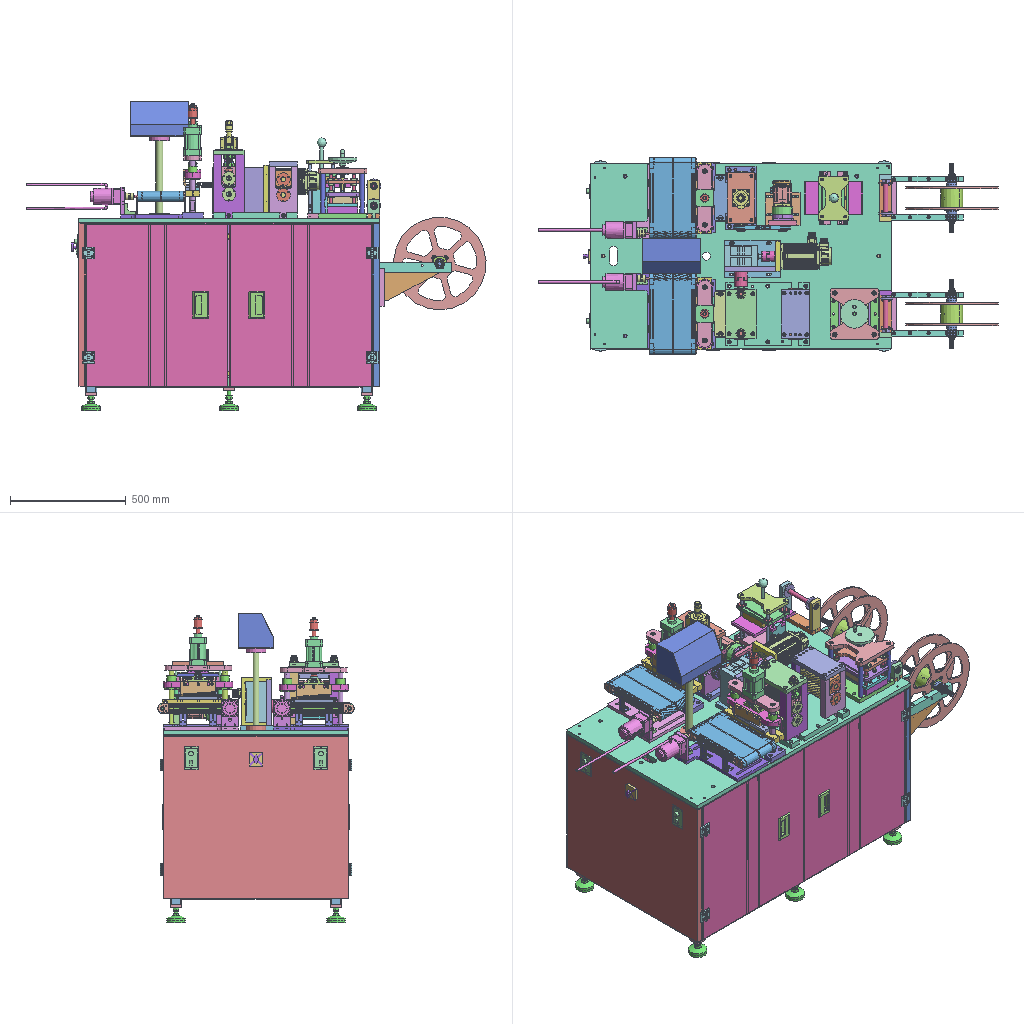Assembly | STEP file | 146 different items | 335 placed | box 1985 x 849 x 1335 mm
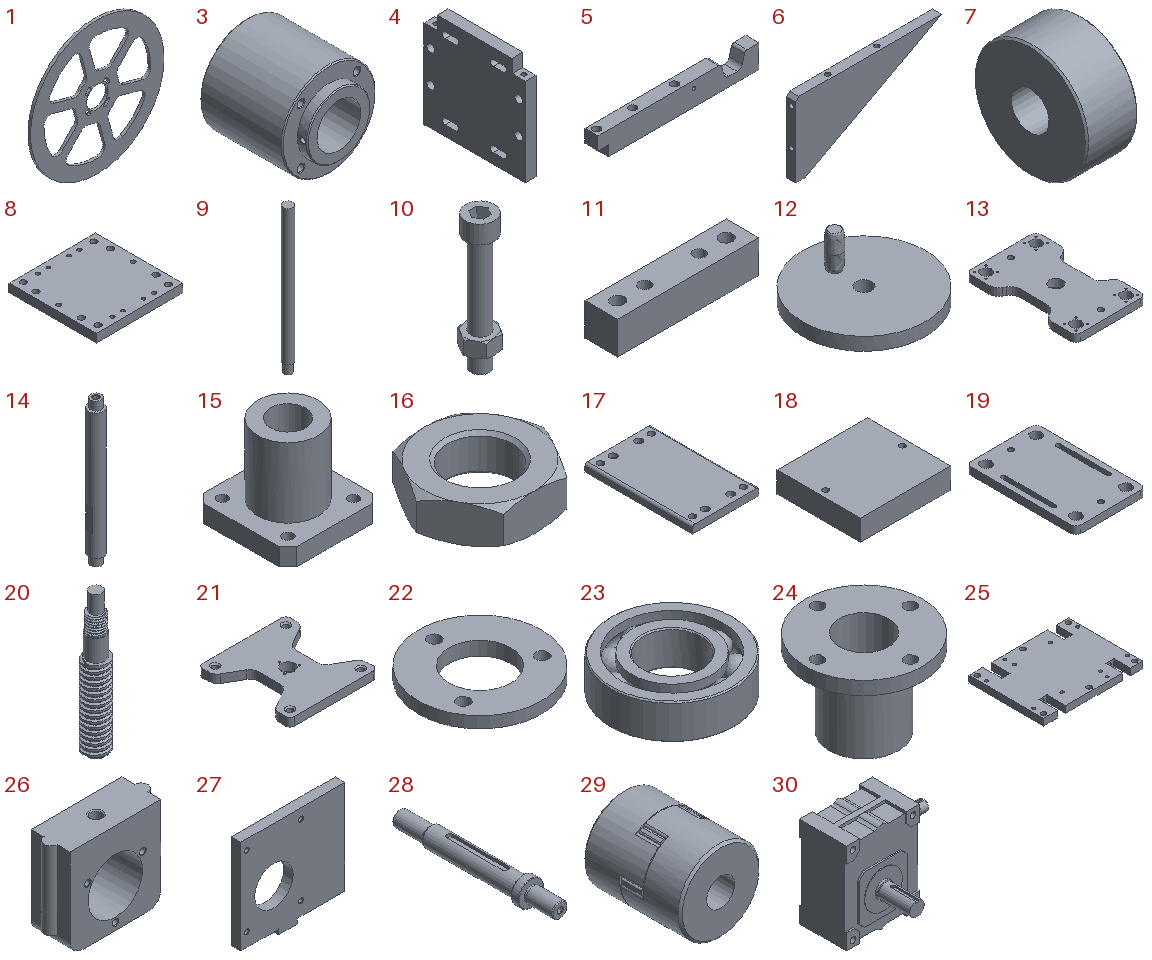Parts list (item | name | quantity | parent item | size | volume):
1 | YBQDJ-FLJ-1 | x4 | in YBQDJ-FLJ | 400 x 8 x 400 mm | 566908 mm3
2 | YBQDJ-FLJ-3 | x2 | in YBQDJ-FLJ | - | -
3 | YBQDJ-FLJ-2 | x2 | in YBQDJ-FLJ | 95 x 103 x 95 mm | 482469 mm3
4 | YBQDJ-FLJ-5 | x2 | in YBQDJ-FLJ | 20 x 190 x 190 mm | 661776 mm3
5 | YBQDJ-FLJ-4 | x4 | in YBQDJ-FLJ | 310 x 25 x 45 mm | 300462 mm3
6 | YBQDJ-FLJ-6 | x4 | in YBQDJ-FLJ | 237.857 x 15 x 120 mm | 224363 mm3
7 | YBQDJ-FLJ-7 | x8 | in YBQDJ-FLJ | 15 x 33 x 33 mm | 11378 mm3
8 | YBQDJ-YL-1 | x1 | in YBQDJ-YL | 210 x 210 x 20 mm | 848713 mm3
9 | YBQDJ-YL-8 | x4 | in YBQDJ-YL | 12 x 12 x 182 mm | 19664 mm3
10 | YBQDJ-YL-13 | x2 | in YBQDJ-YL | 18.475 x 16 x 75 mm | 8074 mm3
11 | YBQDJ-YL-2 | x2 | in YBQDJ-YL | 130 x 30 x 30 mm | 104775 mm3
12 | YBQDJ-YL-10 | x1 | in YBQDJ-YL | 125 x 125 x 70 mm | 226936 mm3
13 | YBQDJ-YL-5 | x1 | in YBQDJ-YL | 140 x 220 x 15 mm | 360572 mm3
14 | YBQDJ-YL-9 | x4 | in YBQDJ-YL | 20 x 20 x 198 mm | 57396 mm3
15 | YBQDJ-YL-14 | x8 | in YBQDJ-YL | 32 x 32 x 30 mm | 10494 mm3
16 | YBQDJ-YL-12 | x1 | in YBQDJ-YL | 24.249 x 21 x 7 mm | 1795 mm3
17 | YBQDJ-YL-3 | x1 | in YBQDJ-YL | 130 x 210 x 15 mm | 393827 mm3
18 | YBQDJ-YL-7 | x1 | in YBQDJ-YL | 130 x 120 x 30 mm | 464984 mm3
19 | YBQDJ-YL-4 | x1 | in YBQDJ-YL | 140 x 220 x 15 mm | 408740 mm3
20 | YBQDJ-YL-11 | x1 | in YBQDJ-YL | 20 x 20 x 118 mm | 24858 mm3
21 | YBQDJ-YL-6 | x1 | in YBQDJ-YL | 210 x 220 x 20 mm | 625567 mm3
22 | YBQDJ-YL-15 | x2 | in YBQDJ-YL | 54 x 54 x 6 mm | 8414 mm3
23 | YBQDJ-YL-16 | x2 | in YBQDJ-YL | 32 x 32 x 9 mm | 3911 mm3
24 | YBQDJ-YL-17 | x1 | in YBQDJ-YL | 44 x 44 x 32 mm | 13018 mm3
25 | YBQDJ-YB-1 | x1 | in YBQDJ-YB | 360 x 270 x 24 mm | 2084097 mm3
26 | YBQDJ-YB-3 | x2 | in YBQDJ-YB | 80 x 30 x 70 mm | 107518 mm3
27 | YBQDJ-YB-18 | x1 | in YBQDJ-YB | 220 x 20 x 210 mm | 773333 mm3
28 | YBQDJ-YB-16 | x1 | in YBQDJ-YB | 33 x 210 x 33 mm | 88192 mm3
29 | YBQDJ-YB-17 | x1 | in YBQDJ-YB | 55 x 66 x 55 mm | 122440 mm3
30 | YBQDJ-YB-20 | x1 | in YBQDJ-YB | 193 x 155 x 174 mm | 2083887 mm3
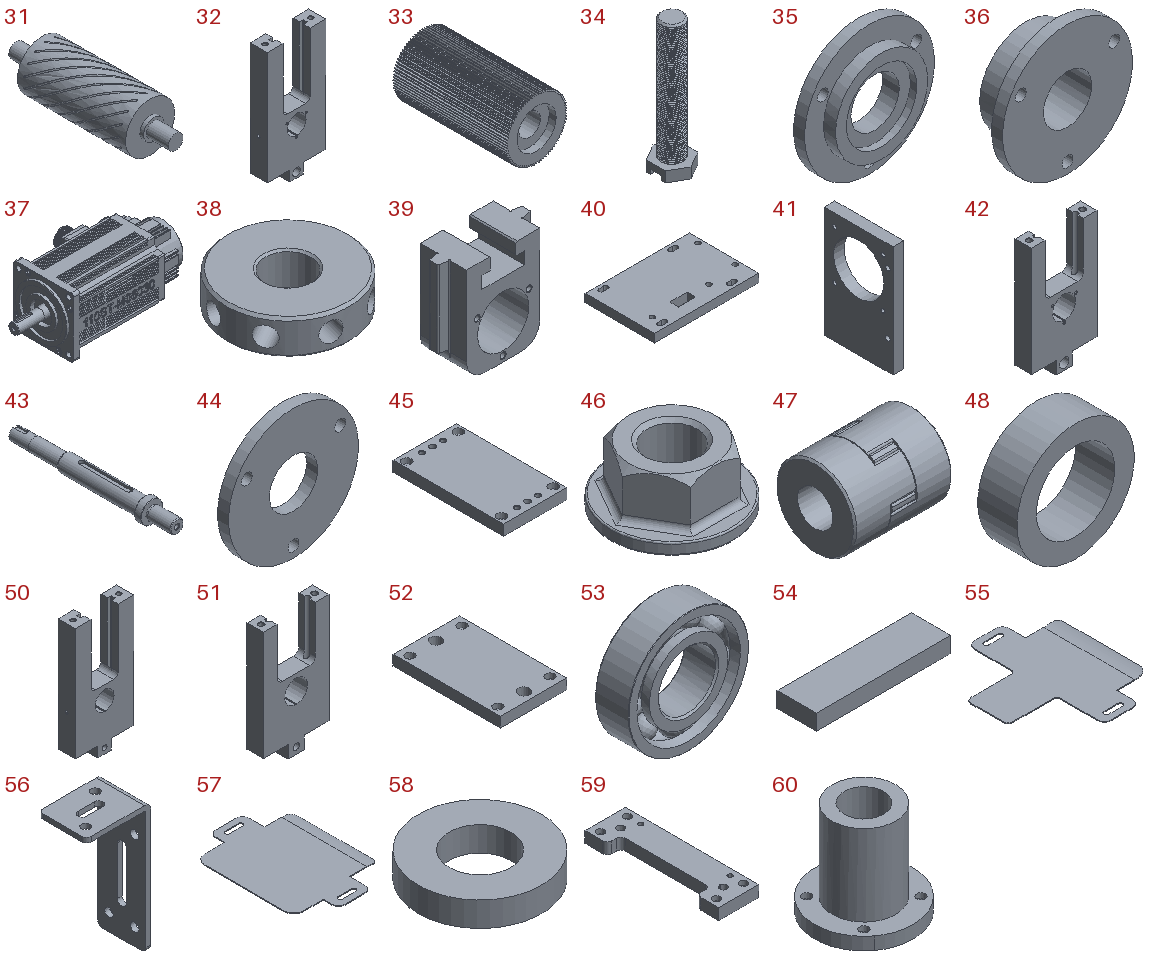31 | YBQDJ-YB-5 | x2 | in YBQDJ-YB | 68.992 x 218 x 68.953 mm | 543044 mm3
32 | YBQDJ-YB-6 | x1 | in YBQDJ-YB | 130 x 38 x 273 mm | 843391 mm3
33 | YBQDJ-YB-15 | x2 | in YBQDJ-YB | 69.832 x 130 x 69.818 mm | 396551 mm3
34 | YBQDJ-YB-8 | x2 | in YBQDJ-YB | 30 x 34.641 x 119.5 mm | 39653 mm3
35 | YBQDJ-YB-13 | x2 | in YBQDJ-YB | 59 x 10.5 x 59 mm | 15659 mm3
36 | YBQDJ-YB-12 | x2 | in YBQDJ-YB | 59 x 19 x 59 mm | 24092 mm3
37 | YBQDJ-YB-22 | x1 | in YBQDJ-YB | 275 x 158 x 110 mm | 3118501 mm3
38 | YBQDJ-YB-9 | x4 | in YBQDJ-YB | 50 x 50 x 14 mm | 18346 mm3
39 | YBQDJ-YB-7 | x2 | in YBQDJ-YB | 76 x 38 x 80 mm | 112101 mm3
40 | YBQDJ-YB-19 | x1 | in YBQDJ-YB | 240 x 160 x 19 mm | 686478 mm3
41 | YBQDJ-YB-21 | x1 | in YBQDJ-YB | 20 x 130 x 210 mm | 393461 mm3
42 | YBQDJ-YB-2 | x1 | in YBQDJ-YB | 120 x 30 x 223 mm | 466414 mm3
43 | YBQDJ-YB-11 | x1 | in YBQDJ-YB | 33 x 245 x 33 mm | 98573 mm3
44 | YBQDJ-YB-14 | x4 | in YBQDJ-YB | 59 x 5 x 59 mm | 11475 mm3
45 | YBQDJ-YB-4 | x1 | in YBQDJ-YB | 120 x 210 x 20 mm | 483124 mm3
46 | YBQDJ-YB-10 | x2 | in YBQDJ-YB | 42.8 x 42.8 x 20 mm | 13331 mm3
47 | YBQDJ-YB-23 | x1 | in YBQDJ-YB | 55 x 45 x 45 mm | 72571 mm3
48 | YBQDJ-YB-24 | x2 | in YBQDJ-YB | 30 x 10 x 30 mm | 3895 mm3
49 | YBQDJ-YB-25 | x1 | in YBQDJ-YB | - | -
50 | YBQDJ-YB-27 | x1 | in YBQDJ-YB | 130 x 38 x 273 mm | 843391 mm3
51 | YBQDJ-YB-26 | x1 | in YBQDJ-YB | 120 x 30 x 223 mm | 466414 mm3
52 | YBQDJ-YB-28 | x1 | in YBQDJ-YB | 130 x 210 x 20 mm | 518119 mm3
53 | YBQDJ-YB-29 | x16 | in YBQDJ-YB | 42 x 12 x 42 mm | 8686 mm3
54 | YBQDJ-YB-30 | x2 | in YBQDJ-YB | 34.5 x 10 x 4 mm | 1380 mm3
55 | YBQDJ-YB-34 | x1 | in YBQDJ-YB | 164.076 x 196 x 5.026 mm | 23129 mm3
56 | YBQDJ-YB-31 | x2 | in YBQDJ-YB | 40 x 30 x 80 mm | 9225 mm3
57 | YBQDJ-YB-32 | x1 | in YBQDJ-YB | 139.076 x 196 x 5.026 mm | 26086 mm3
58 | YBQDJ-YB-33 | x2 | in YBQDJ-YB | 20 x 20 x 4 mm | 942.478 mm3
59 | YBQDJ-QD-1 | x2 | in YBQDJ-QD-BD, YBQDJ-QD-PD | 90 x 300 x 25 mm | 495978 mm3
60 | YBQDJ-QD-7 | x4 | in YBQDJ-QD-BD, YBQDJ-QD-PD | 62 x 62 x 59 mm | 57722 mm3
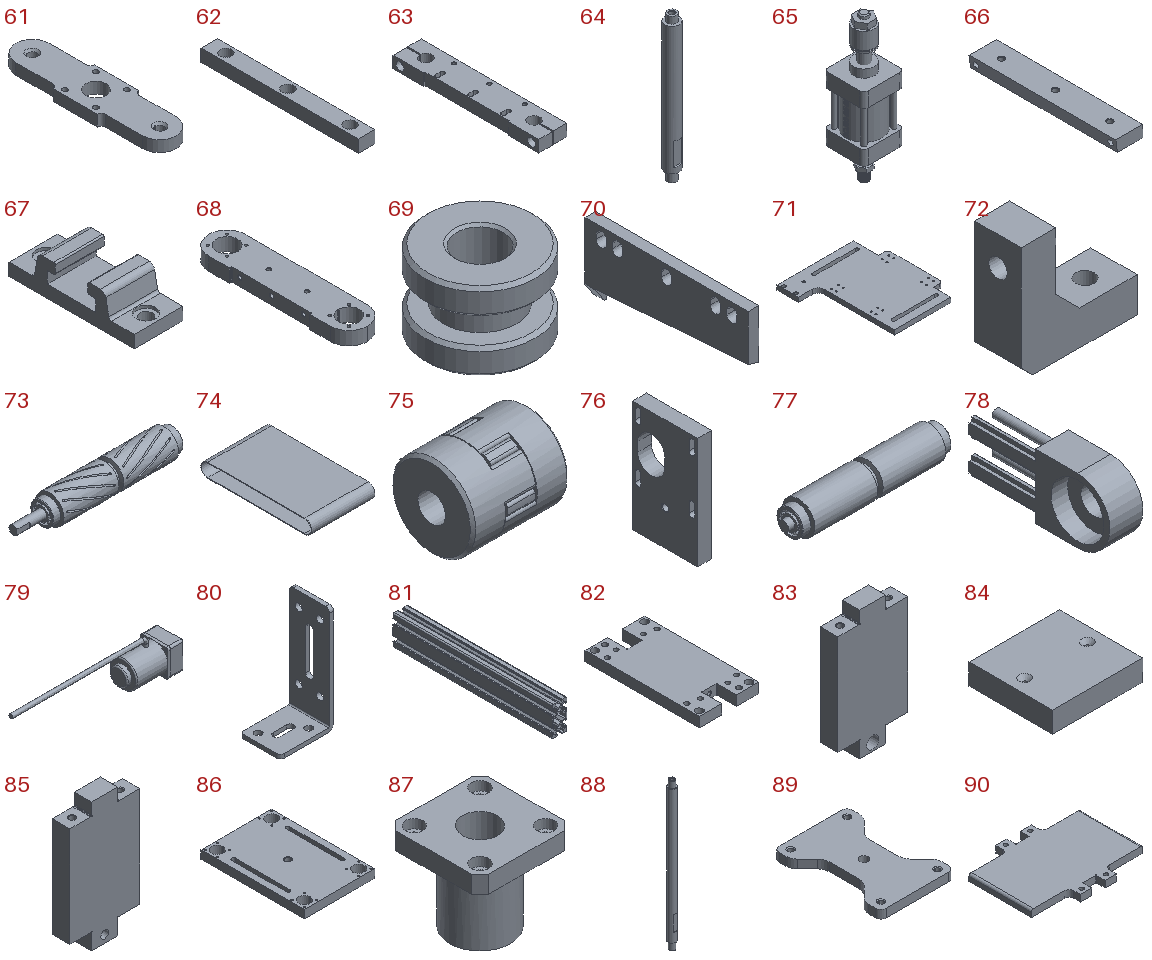61 | YBQDJ-QD-10 | x2 | in YBQDJ-QD-BD, YBQDJ-QD-PD | 75 x 290 x 20 mm | 318824 mm3
62 | YBQDJ-QD-4 | x2 | in YBQDJ-QD-BD, YBQDJ-QD-PD | 20 x 190 x 15 mm | 51822 mm3
63 | YBQDJ-QD-3 | x2 | in YBQDJ-QD-BD, YBQDJ-QD-PD | 60 x 310 x 25 mm | 397510 mm3
64 | YBQDJ-QD-2 | x2 | in YBQDJ-QD-BD | 25 x 25 x 254 mm | 111454 mm3
65 | YBQDJ-QD-11 | x2 | in YBQDJ-QD-BD, YBQDJ-QD-PD | 75 x 75 x 272 mm | 699847 mm3
66 | YBQDJ-QD-5 | x2 | in YBQDJ-QD-BD, YBQDJ-QD-PD | 35 x 190 x 15 mm | 92776 mm3
67 | YBQDJ-QD-8 | x2 | in YBQDJ-QD-BD, YBQDJ-QD-PD | 35 x 90 x 25 mm | 38677 mm3
68 | YBQDJ-QD-6 | x2 | in YBQDJ-QD-BD, YBQDJ-QD-PD | 70 x 300 x 25 mm | 414235 mm3
69 | YBQDJ-QD-9 | x2 | in YBQDJ-QD-BD, YBQDJ-QD-PD | 34 x 34 x 24 mm | 13509 mm3
70 | YBQDJ-QD-12 | x2 | in YBQDJ-QD-BD, YBQDJ-QD-PD | 10 x 150 x 65 mm | 69081 mm3
71 | YBQDJ-SSJ-1 | x1 | in YBQDJ-SSJ-BD | 280 x 320 x 15 mm | 982860 mm3
72 | YBQDJ-SSJ-8 | x2 | in YBQDJ-SSJ-BD, YBQD-SSJ-PD_MODEL | 50 x 20 x 50 mm | 24742 mm3
73 | YBQDJ-SSJ-7 | x2 | in YBQDJ-SSJ-BD, YBQD-SSJ-PD_MODEL | 227 x 40.957 x 41.285 mm | 212732 mm3
74 | YBQDJ-SSJ-3 | x2 | in YBQDJ-SSJ-BD, YBQD-SSJ-PD_MODEL | 200 x 350 x 44 mm | 311989 mm3
75 | YBQDJ-SSJ-11 | x2 | in YBQDJ-SSJ-BD, YBQD-SSJ-PD_MODEL | 35 x 30 x 30 mm | 20965 mm3
76 | YBQDJ-SSJ-9 | x2 | in YBQDJ-SSJ-BD, YBQD-SSJ-PD_MODEL | 15 x 70 x 120 mm | 105388 mm3
77 | YBQDJ-SSJ-6 | x2 | in YBQDJ-SSJ-BD, YBQD-SSJ-PD_MODEL | 196 x 40 x 40 mm | 211425 mm3
78 | YBQDJ-SSJ-4 | x8 | in YBQDJ-SSJ-BD, YBQD-SSJ-PD_MODEL | 20 x 85 x 39 mm | 27065 mm3
79 | YBQDJ-SSJ-10 | x2 | in YBQDJ-SSJ-BD, YBQD-SSJ-PD_MODEL | - | -
80 | YBQDJ-SSJ-2 | x8 | in YBQDJ-SSJ-BD, YBQD-SSJ-PD_MODEL | 40 x 30 x 80 mm | 9225 mm3
81 | YBQDJ-SSJ-5 | x4 | in YBQDJ-SSJ-BD, YBQD-SSJ-PD_MODEL | 20 x 215 x 40 mm | 63524 mm3
82 | YBQDJ-YY-1 | x1 | in YBQDJ-YY | 120 x 230 x 20 mm | 476492 mm3
83 | YBQDJ-YY-3 | x1 | in YBQDJ-YY | 80 x 20 x 148 mm | 197857 mm3
84 | YBQDJ-YY-5 | x1 | in YBQDJ-YY | 130 x 120 x 30 mm | 465920 mm3
85 | YBQDJ-YY-2 | x1 | in YBQDJ-YY | 80 x 20 x 148 mm | 197857 mm3
86 | YBQDJ-YY-7 | x1 | in YBQDJ-YY | 130 x 190 x 15 mm | 325427 mm3
87 | YBQDJ-YY-6 | x4 | in YBQDJ-YY | 32 x 32 x 30 mm | 10494 mm3
88 | YBQDJ-YY-10 | x4 | in YBQDJ-YY | 12 x 12 x 237 mm | 24995 mm3
89 | YBQDJ-YY-8 | x1 | in YBQDJ-YY | 130 x 190 x 15 mm | 272574 mm3
90 | YBQDJ-YY-4 | x1 | in YBQDJ-YY | 250 x 190 x 15 mm | 563148 mm3
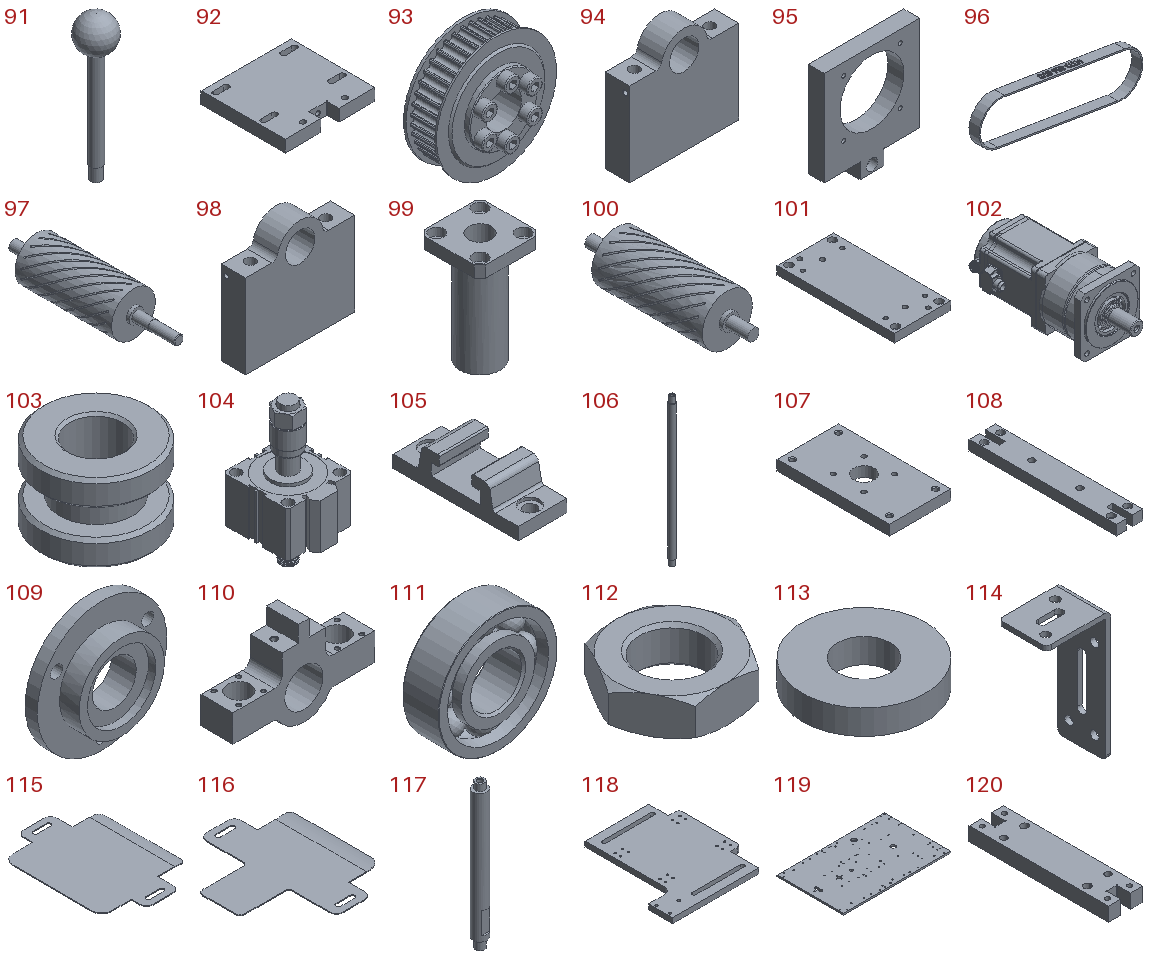91 | YBQDJ-YY-9 | x1 | in YBQDJ-YY | 40 x 40 x 166 mm | 52339 mm3
92 | YBQDJ-PD-1 | x1 | in YBQDJ-PD_MODEL | 150 x 140 x 20 mm | 385255 mm3
93 | YBQDJ-PD-4 | x2 | in YBQDJ-PD_MODEL | 67 x 28.5 x 67 mm | 55543 mm3
94 | YBQDJ-PD-7 | x1 | in YBQDJ-PD_MODEL | 130 x 29.2 x 127.5 mm | 362195 mm3
95 | YBQDJ-PD-3 | x1 | in YBQDJ-PD_MODEL | 120 x 20 x 138 mm | 191169 mm3
96 | YBQDJ-PD-5 | x1 | in YBQDJ-PD_MODEL | 245.482 x 15 x 95 mm | 17074 mm3
97 | YBQDJ-PD-9 | x1 | in YBQDJ-PD_MODEL | 68.992 x 253 x 68.953 mm | 537694 mm3
98 | YBQDJ-PD-8 | x1 | in YBQDJ-PD_MODEL | 130 x 29.2 x 127.5 mm | 362195 mm3
99 | YBQDJ-PD-11 | x4 | in YBQDJ-PD_MODEL | 32 x 32 x 57 mm | 16408 mm3
100 | YBQDJ-PD-10 | x1 | in YBQDJ-PD_MODEL | 68.992 x 218 x 68.953 mm | 532441 mm3
101 | YBQDJ-PD-6 | x1 | in YBQDJ-PD_MODEL | 130 x 270 x 19 mm | 640127 mm3
102 | YBQDJ-PD-2 | x1 | in YBQDJ-PD_MODEL | - | 675014 mm3
103 | YBQDJ-PD-16 | x1 | in YBQDJ-PD_MODEL | 34 x 34 x 24 mm | 12336 mm3
104 | YBQDJ-PD-15 | x1 | in YBQDJ-PD_MODEL | 76 x 84.5 x 162 mm | 333527 mm3
105 | YBQDJ-PD-17 | x1 | in YBQDJ-PD_MODEL | 35 x 90 x 25 mm | 38677 mm3
106 | YBQDJ-PD-13 | x4 | in YBQDJ-PD_MODEL | 12 x 12 x 284 mm | 30280 mm3
107 | YBQDJ-PD-14 | x1 | in YBQDJ-PD_MODEL | 120 x 220 x 20 mm | 489101 mm3
108 | YBQDJ-PD-18 | x1 | in YBQDJ-PD_MODEL | 40 x 220 x 15 mm | 117739 mm3
109 | YBQDJ-PD-19 | x4 | in YBQDJ-PD_MODEL | 53 x 13 x 53 mm | 13997 mm3
110 | YBQDJ-PD-12 | x2 | in YBQDJ-PD_MODEL | 130 x 29.2 x 80 mm | 97793 mm3
111 | YBQDJ-PD-20 | x8 | in YBQDJ-PD_MODEL | 35 x 11 x 35 mm | 5907 mm3
112 | YBQDJ-PD-21 | x1 | in YBQDJ-PD_MODEL | 31.177 x 27 x 9 mm | 3802 mm3
113 | YBQDJ-PD-24 | x2 | in YBQDJ-PD_MODEL | 20 x 20 x 4 mm | 1030 mm3
114 | YBQDJ-PD-25 | x2 | in YBQDJ-PD_MODEL | 40 x 30 x 80 mm | 9225 mm3
115 | YBQDJ-PD-22 | x1 | in YBQDJ-PD_MODEL | 139.076 x 196 x 5.026 mm | 26086 mm3
116 | YBQDJ-PD-23 | x1 | in YBQDJ-PD_MODEL | 164.076 x 196 x 5.026 mm | 23129 mm3
117 | YBQDJ-QD-PD-2 | x2 | in YBQDJ-QD-PD | 25 x 25 x 264 mm | 116363 mm3
118 | YBQDJ-SSJ-PD-1 | x1 | in YBQD-SSJ-PD_MODEL | 280 x 320 x 15 mm | 982860 mm3
119 | YBQDJ-Large plate | x1 | in Pressure-wave cutting all-in-one machine general unit | 1300 x 800 x 20 mm | 20508106 mm3
120 | YBQDJ-DX-1 | x2 | in YBQDJ-DX-PD_MODEL, YBQDJ-DX-BD_MODEL | 50 x 200 x 20 mm | 177964 mm3
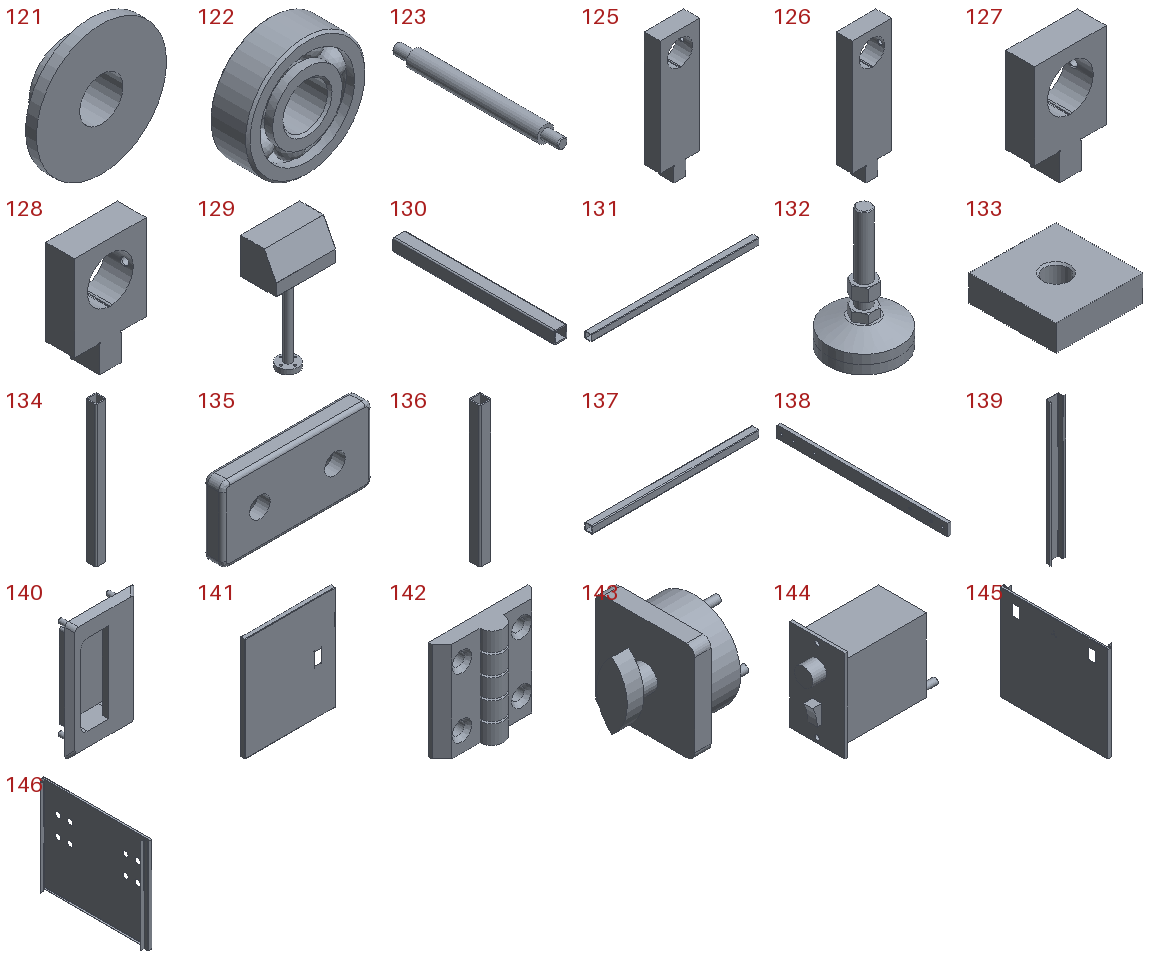121 | YBQDJ-DX-3 | x4 | in YBQDJ-DX-PD_MODEL, YBQDJ-DX-BD_MODEL | 60 x 16 x 60 mm | 19587 mm3
122 | YBQDJ-DX-6 | x8 | in YBQDJ-DX-PD_MODEL, YBQDJ-DX-BD_MODEL | 32 x 10 x 32 mm | 4745 mm3
123 | YBQDJ-DX-4 | x2 | in YBQDJ-DX-PD_MODEL, YBQDJ-DX-BD_MODEL | 20 x 200 x 20 mm | 54352 mm3
124 | YBQDJ-DX-5 | x2 | in YBQDJ-DX-PD_MODEL, YBQDJ-DX-BD_MODEL | - | -
125 | YBQDJ-DX-2 | x1 | in YBQDJ-DX-PD_MODEL | 50 x 20 x 164 mm | 134384 mm3
126 | YBQDJ-DX-7 | x1 | in YBQDJ-DX-PD_MODEL | 50 x 20 x 164 mm | 134384 mm3
127 | YBQDJ-DX-BD-2 | x1 | in YBQDJ-DX-BD_MODEL | 50 x 20 x 79 mm | 49384 mm3
128 | YBQDJ-DX-BD-7 | x1 | in YBQDJ-DX-BD_MODEL | 50 x 20 x 79 mm | 49384 mm3
129 | Touch screen assembly | x1 | in Pressure-wave cutting all-in-one machine general unit | 250 x 150 x 505 mm | 675168 mm3
130 | 50x50x640 | x6 | in YBQDJ-JJ_MODEL | 50 x 640 x 50 mm | 562265 mm3
131 | 50x50x1240 | x2 | in YBQDJ-JJ_MODEL | 1240 x 50 x 50 mm | 1089389 mm3
132 | Foot cup | x6 | in 50x50x680_MODEL, 50x50x1140_MODEL | 80 x 80 x 135 mm | 154518 mm3
133 | Pad block | x6 | in 50x50x680_MODEL, 50x50x1140_MODEL | 50 x 50 x 15 mm | 35145 mm3
134 | SOLID | x4 | in 50x50x680_MODEL | 50 x 50 x 680 mm | 597407 mm3
135 | Door magnet | x4 | in 50x50x610_MODEL | 40 x 5 x 20 mm | 3632 mm3
136 | SOLID | x2 | in 50x50x610_MODEL | 50 x 50 x 610 mm | 535909 mm3
137 | SOLID | x2 | in 50x50x1140_MODEL | 1140 x 50 x 50 mm | 1000530 mm3
138 | Crossbeam | x2 | in YBQDJ-JJ_MODEL | 15 x 730 x 50 mm | 541334 mm3
139 | Reinforcing rib | x4 | in YBQDJ-BJ-1_MODEL | 80 x 26.7 x 696 mm | 106400 mm3
140 | Handle | x4 | in YBQDJ-BJ-1_MODEL | 69 x 21 x 119 mm | 44051 mm3
141 | SOLID | x4 | in YBQDJ-BJ-1_MODEL | 615 x 30 x 705 mm | 627775 mm3
142 | Hinge | x8 | in YBQDJ-BJ_MODEL | 50 x 12.7 x 49.8 mm | 17221 mm3
143 | Power switch | x1 | in YBQDJ-BJ-2_MODEL | 64 x 60 x 60 mm | 180692 mm3
144 | Speed control panel | x2 | in YBQDJ-BJ-2_MODEL | 122.5 x 60 x 100 mm | 404808 mm3
145 | SOLID | x1 | in YBQDJ-BJ-2_MODEL | 55 x 800 x 705 mm | 825706 mm3
146 | YBQDJ-BJ-3 | x1 | in YBQDJ-BJ_MODEL | 55 x 800 x 705 mm | 823970 mm3
Placements (level | parent | child | x y z in mm | rotation matrix by rows), first 235 of 362 lines:
1 | Pressure-wave cutting all-in-one machine general unit | YBQDJ-FLJ | 0.0 0.0 0.0 | 1 0 0 0 1 0 0 0 1
2 | YBQDJ-FLJ | YBQDJ-FLJ-1 | 0.0 0.0 0.0 | 1 0 0 0 1 0 0 0 1
2 | YBQDJ-FLJ | YBQDJ-FLJ-3 | 0.0 0.0 0.0 | 1 0 0 0 1 0 0 0 1
2 | YBQDJ-FLJ | YBQDJ-FLJ-2 | 0.0 0.0 0.0 | 1 0 0 0 1 0 0 0 1
2 | YBQDJ-FLJ | YBQDJ-FLJ-1 | 0.0 91.0 0.0 | 1 0 0 0 1 0 0 0 1
2 | YBQDJ-FLJ | YBQDJ-FLJ-5 | 0.0 0.0 0.0 | 1 0 0 0 1 0 0 0 1
2 | YBQDJ-FLJ | YBQDJ-FLJ-4 | 0.0 0.0 0.0 | 1 0 0 0 1 0 0 0 1
2 | YBQDJ-FLJ | YBQDJ-FLJ-6 | 0.0 0.0 0.0 | 1 0 0 0 1 0 0 0 1
2 | YBQDJ-FLJ | YBQDJ-FLJ-6 | 0.0 165.0 0.0 | 1 0 0 0 1 0 0 0 1
2 | YBQDJ-FLJ | YBQDJ-FLJ-4 | 0.0 165.0 0.0 | 1 0 0 0 1 0 0 0 1
2 | YBQDJ-FLJ | YBQDJ-FLJ-7 | -0.0 90.0 -140.0 | 1 0 0 0 1 0 0 0 1
2 | YBQDJ-FLJ | YBQDJ-FLJ-7 | -0.0 90.0 -0.0 | 1 0 0 0 1 0 0 0 1
2 | YBQDJ-FLJ | YBQDJ-FLJ-7 | 0.0 0.0 0.0 | 1 0 0 0 1 0 0 0 1
2 | YBQDJ-FLJ | YBQDJ-FLJ-7 | 0.0 0.0 -140.0 | 1 0 0 0 1 0 0 0 1
1 | Pressure-wave cutting all-in-one machine general unit | YBQDJ-FLJ | 0.0 500.0 0.0 | 1 0 0 0 1 0 0 0 1
2 | YBQDJ-FLJ | YBQDJ-FLJ-1 | 0.0 0.0 0.0 | 1 0 0 0 1 0 0 0 1
2 | YBQDJ-FLJ | YBQDJ-FLJ-3 | 0.0 0.0 0.0 | 1 0 0 0 1 0 0 0 1
2 | YBQDJ-FLJ | YBQDJ-FLJ-2 | 0.0 0.0 0.0 | 1 0 0 0 1 0 0 0 1
2 | YBQDJ-FLJ | YBQDJ-FLJ-1 | 0.0 91.0 0.0 | 1 0 0 0 1 0 0 0 1
2 | YBQDJ-FLJ | YBQDJ-FLJ-5 | 0.0 0.0 0.0 | 1 0 0 0 1 0 0 0 1
2 | YBQDJ-FLJ | YBQDJ-FLJ-4 | 0.0 0.0 0.0 | 1 0 0 0 1 0 0 0 1
2 | YBQDJ-FLJ | YBQDJ-FLJ-6 | 0.0 0.0 0.0 | 1 0 0 0 1 0 0 0 1
2 | YBQDJ-FLJ | YBQDJ-FLJ-6 | 0.0 165.0 0.0 | 1 0 0 0 1 0 0 0 1
2 | YBQDJ-FLJ | YBQDJ-FLJ-4 | 0.0 165.0 0.0 | 1 0 0 0 1 0 0 0 1
2 | YBQDJ-FLJ | YBQDJ-FLJ-7 | -0.0 90.0 -140.0 | 1 0 0 0 1 0 0 0 1
2 | YBQDJ-FLJ | YBQDJ-FLJ-7 | -0.0 90.0 -0.0 | 1 0 0 0 1 0 0 0 1
2 | YBQDJ-FLJ | YBQDJ-FLJ-7 | 0.0 0.0 0.0 | 1 0 0 0 1 0 0 0 1
2 | YBQDJ-FLJ | YBQDJ-FLJ-7 | 0.0 0.0 -140.0 | 1 0 0 0 1 0 0 0 1
1 | Pressure-wave cutting all-in-one machine general unit | YBQDJ-YL | 0.0 0.0 0.0 | 1 0 0 0 1 0 0 0 1
2 | YBQDJ-YL | YBQDJ-YL-1 | 0.0 0.0 0.0 | 1 0 0 0 1 0 0 0 1
2 | YBQDJ-YL | YBQDJ-YL-8 | 0.0 0.0 0.0 | 1 0 0 0 1 0 0 0 1
2 | YBQDJ-YL | YBQDJ-YL-13 | 0.0 0.0 0.0 | 1 0 0 0 1 0 0 0 1
2 | YBQDJ-YL | YBQDJ-YL-2 | 0.0 0.0 0.0 | 1 0 0 0 1 0 0 0 1
2 | YBQDJ-YL | YBQDJ-YL-10 | 0.0 0.0 0.0 | 1 0 0 0 1 0 0 0 1
2 | YBQDJ-YL | YBQDJ-YL-5 | 0.0 0.0 0.0 | 1 0 0 0 1 0 0 0 1
2 | YBQDJ-YL | YBQDJ-YL-9 | 0.0 0.0 0.0 | 1 0 0 0 1 0 0 0 1
2 | YBQDJ-YL | YBQDJ-YL-14 | 0.0 0.0 0.0 | 1 0 0 0 1 0 0 0 1
2 | YBQDJ-YL | YBQDJ-YL-12 | 0.0 0.0 0.5 | 1 0 0 0 1 0 0 0 1
2 | YBQDJ-YL | YBQDJ-YL-3 | 0.0 0.0 0.0 | 1 0 0 0 1 0 0 0 1
2 | YBQDJ-YL | YBQDJ-YL-7 | 0.0 0.0 0.0 | 1 0 0 0 1 0 0 0 1
2 | YBQDJ-YL | YBQDJ-YL-4 | 0.0 0.0 0.0 | 1 0 0 0 1 0 0 0 1
2 | YBQDJ-YL | YBQDJ-YL-11 | 0.0 0.0 0.0 | 1 0 0 0 1 0 0 0 1
2 | YBQDJ-YL | YBQDJ-YL-6 | 0.0 0.0 0.0 | 1 0 0 0 1 0 0 0 1
2 | YBQDJ-YL | YBQDJ-YL-2 | 0.0 180.0 0.0 | 1 0 0 0 1 0 0 0 1
2 | YBQDJ-YL | YBQDJ-YL-14 | 100.0 0.0 0.0 | 1 0 0 0 1 0 0 0 1
2 | YBQDJ-YL | YBQDJ-YL-14 | 100.0 180.0 0.0 | 1 0 0 0 1 0 0 0 1
2 | YBQDJ-YL | YBQDJ-YL-14 | 0.0 180.0 0.0 | 1 0 0 0 1 0 0 0 1
2 | YBQDJ-YL | YBQDJ-YL-14 | 613.0 0.0 260.0 | -1 0 0 0 1 0 0 0 -1
2 | YBQDJ-YL | YBQDJ-YL-14 | 513.0 0.0 260.0 | -1 0 0 0 1 0 0 0 -1
2 | YBQDJ-YL | YBQDJ-YL-14 | 613.0 180.0 260.0 | -1 0 0 0 1 0 0 0 -1
2 | YBQDJ-YL | YBQDJ-YL-14 | 513.0 180.0 260.0 | -1 0 0 0 1 0 0 0 -1
2 | YBQDJ-YL | YBQDJ-YL-13 | 0.0 180.0 0.0 | 1 0 0 0 1 0 0 0 1
2 | YBQDJ-YL | YBQDJ-YL-8 | 100.0 0.0 0.0 | 1 0 0 0 1 0 0 0 1
2 | YBQDJ-YL | YBQDJ-YL-8 | 0.0 180.0 0.0 | 1 0 0 0 1 0 0 0 1
2 | YBQDJ-YL | YBQDJ-YL-8 | 100.0 180.0 0.0 | 1 0 0 0 1 0 0 0 1
2 | YBQDJ-YL | YBQDJ-YL-9 | 170.0 0.0 0.0 | 1 0 0 0 1 0 0 0 1
2 | YBQDJ-YL | YBQDJ-YL-9 | 170.0 180.0 0.0 | 1 0 0 0 1 0 0 0 1
2 | YBQDJ-YL | YBQDJ-YL-9 | 0.0 180.0 0.0 | 1 0 0 0 1 0 0 0 1
2 | YBQDJ-YL | YBQDJ-YL-15 | 0.0 0.0 0.0 | 1 0 0 0 1 0 0 0 1
2 | YBQDJ-YL | YBQDJ-YL-16 | 0.0 0.0 0.0 | 1 0 0 0 1 0 0 0 1
2 | YBQDJ-YL | YBQDJ-YL-17 | 0.0 0.0 0.0 | 1 0 0 0 1 0 0 0 1
2 | YBQDJ-YL | YBQDJ-YL-16 | 0.0 0.0 9.0 | 1 0 0 0 1 0 0 0 1
2 | YBQDJ-YL | YBQDJ-YL-15 | 613.0 0.0 408.0 | -1 0 0 0 1 0 0 0 -1
1 | Pressure-wave cutting all-in-one machine general unit | YBQDJ-YB | 0.0 0.0 0.0 | 1 0 0 0 1 0 0 0 1
2 | YBQDJ-YB | YBQDJ-YB-1 | 0.0 0.0 0.0 | 1 0 0 0 1 0 0 0 1
2 | YBQDJ-YB | YBQDJ-YB-3 | 0.0 0.0 0.0 | 1 0 0 0 1 0 0 0 1
2 | YBQDJ-YB | YBQDJ-YB-18 | 0.0 0.0 0.0 | 1 0 0 0 1 0 0 0 1
2 | YBQDJ-YB | YBQDJ-YB-16 | 0.0 0.0 0.0 | 1 0 0 0 1 0 0 0 1
2 | YBQDJ-YB | YBQDJ-YB-17 | 0.0 0.0 0.0 | 1 0 0 0 1 0 0 0 1
2 | YBQDJ-YB | YBQDJ-YB-20 | 0.0 0.0 0.0 | 1 0 0 0 1 0 0 0 1
2 | YBQDJ-YB | YBQDJ-YB-5 | 0.0 0.0 0.0 | 1 0 0 0 1 0 0 0 1
2 | YBQDJ-YB | YBQDJ-YB-6 | 0.0 0.0 0.0 | 1 0 0 0 1 0 0 0 1
2 | YBQDJ-YB | YBQDJ-YB-15 | 0.0 0.0 0.0 | 1 0 0 0 1 0 0 0 1
2 | YBQDJ-YB | YBQDJ-YB-8 | 0.0 0.0 0.0 | 1 0 0 0 1 0 0 0 1
2 | YBQDJ-YB | YBQDJ-YB-13 | 0.0 0.0 0.0 | 1 0 0 0 1 0 0 0 1
2 | YBQDJ-YB | YBQDJ-YB-12 | 0.0 0.0 0.0 | 1 0 0 0 1 0 0 0 1
2 | YBQDJ-YB | YBQDJ-YB-22 | 0.0 0.0 0.0 | 1 0 0 0 1 0 0 0 1
2 | YBQDJ-YB | YBQDJ-YB-9 | 0.0 0.0 0.0 | 1 0 0 0 1 0 0 0 1
2 | YBQDJ-YB | YBQDJ-YB-7 | 0.0 0.0 0.0 | 1 0 0 0 1 0 0 0 1
2 | YBQDJ-YB | YBQDJ-YB-19 | 0.0 0.0 0.0 | 1 0 0 0 1 0 0 0 1
2 | YBQDJ-YB | YBQDJ-YB-21 | 0.0 0.0 0.0 | 1 0 0 0 1 0 0 0 1
2 | YBQDJ-YB | YBQDJ-YB-2 | 0.0 0.0 0.0 | 1 0 0 0 1 0 0 0 1
2 | YBQDJ-YB | YBQDJ-YB-11 | 0.0 0.0 0.0 | 1 0 0 0 1 0 0 0 1
2 | YBQDJ-YB | YBQDJ-YB-14 | 0.0 0.0 0.0 | 1 0 0 0 1 0 0 0 1
2 | YBQDJ-YB | YBQDJ-YB-4 | 0.0 0.0 0.0 | 1 0 0 0 1 0 0 0 1
2 | YBQDJ-YB | YBQDJ-YB-10 | 0.0 0.0 0.0 | 1 0 0 0 1 0 0 0 1
2 | YBQDJ-YB | YBQDJ-YB-23 | 0.0 0.0 0.0 | 1 0 0 0 1 0 0 0 1
2 | YBQDJ-YB | YBQDJ-YB-24 | 0.0 0.0 0.0 | 1 0 0 0 1 0 0 0 1
2 | YBQDJ-YB | YBQDJ-YB-25 | 0.0 0.0 0.0 | 1 0 0 0 1 0 0 0 1
2 | YBQDJ-YB | YBQDJ-YB-27 | 0.0 0.0 0.0 | 1 0 0 0 1 0 0 0 1
2 | YBQDJ-YB | YBQDJ-YB-26 | 0.0 0.0 0.0 | 1 0 0 0 1 0 0 0 1
2 | YBQDJ-YB | YBQDJ-YB-28 | 0.0 0.0 0.0 | 1 0 0 0 1 0 0 0 1
2 | YBQDJ-YB | YBQDJ-YB-29 | 0.0 0.0 0.0 | 1 0 0 0 1 0 0 0 1
2 | YBQDJ-YB | YBQDJ-YB-29 | 0.0 -12.0 0.0 | 1 0 0 0 1 0 0 0 1
2 | YBQDJ-YB | YBQDJ-YB-29 | 0.0 182.0 0.0 | 1 0 0 0 1 0 0 0 1
2 | YBQDJ-YB | YBQDJ-YB-29 | 0.0 170.0 0.0 | 1 0 0 0 1 0 0 0 1
2 | YBQDJ-YB | YBQDJ-YB-29 | 0.0 0.0 67.0 | 1 0 0 0 1 0 0 0 1
2 | YBQDJ-YB | YBQDJ-YB-29 | 0.0 170.0 67.0 | 1 0 0 0 1 0 0 0 1
2 | YBQDJ-YB | YBQDJ-YB-29 | 0.0 182.0 67.0 | 1 0 0 0 1 0 0 0 1
2 | YBQDJ-YB | YBQDJ-YB-5 | 0.0 0.0 67.0 | 1 0 0 0 1 0 0 0 1
2 | YBQDJ-YB | YBQDJ-YB-29 | 0.0 -12.0 67.0 | 1 0 0 0 1 0 0 0 1
2 | YBQDJ-YB | YBQDJ-YB-14 | -0.0 0.0 67.0 | 1 0 0 0 1 0 0 0 1
2 | YBQDJ-YB | YBQDJ-YB-3 | 103.0 -390.0 0.0 | -1 0 0 0 -1 0 0 0 1
2 | YBQDJ-YB | YBQDJ-YB-14 | 103.0 -390.0 0.0 | -1 0 0 0 -1 0 0 0 1
2 | YBQDJ-YB | YBQDJ-YB-14 | 103.0 -390.0 67.0 | -1 0 0 0 -1 0 0 0 1
2 | YBQDJ-YB | YBQDJ-YB-15 | 0.0 0.0 68.3 | 1 0 0 0 1 0 0 0 1
2 | YBQDJ-YB | YBQDJ-YB-29 | -235.0 12.0 3.0 | 1 0 0 0 1 0 0 0 1
2 | YBQDJ-YB | YBQDJ-YB-29 | -235.0 0.0 3.0 | 1 0 0 0 1 0 0 0 1
2 | YBQDJ-YB | YBQDJ-YB-29 | -235.0 0.0 71.3 | 1 0 0 0 1 0 0 0 1
2 | YBQDJ-YB | YBQDJ-YB-29 | -235.0 12.0 71.3 | 1 0 0 0 1 0 0 0 1
2 | YBQDJ-YB | YBQDJ-YB-12 | -0.0 0.0 68.3 | 1 0 0 0 1 0 0 0 1
2 | YBQDJ-YB | YBQDJ-YB-9 | 0.0 0.0 36.7 | 1 0 0 0 1 0 0 0 1
2 | YBQDJ-YB | YBQDJ-YB-7 | -367 -390 -0.0 | -1 1e-06 0 -1e-06 -1 0 0 0 1
2 | YBQDJ-YB | YBQDJ-YB-9 | 0.0 172.0 36.7 | 1 0 0 0 1 0 0 0 1
2 | YBQDJ-YB | YBQDJ-YB-8 | 0.0 172.0 0.0 | 1 0 0 0 1 0 0 0 1
2 | YBQDJ-YB | YBQDJ-YB-9 | 0.0 172.0 0.0 | 1 0 0 0 1 0 0 0 1
2 | YBQDJ-YB | YBQDJ-YB-10 | 0.0 172.0 0.0 | 1 0 0 0 1 0 0 0 1
2 | YBQDJ-YB | YBQDJ-YB-24 | 0.0 0.0 68.3 | 1 0 0 0 1 0 0 0 1
2 | YBQDJ-YB | YBQDJ-YB-29 | -235.0 166.5 3.0 | 1 0 0 0 1 0 0 0 1
2 | YBQDJ-YB | YBQDJ-YB-29 | -235.0 178.5 3.0 | 1 0 0 0 1 0 0 0 1
2 | YBQDJ-YB | YBQDJ-YB-13 | 0.0 0.0 68.3 | 1 0 0 0 1 0 0 0 1
2 | YBQDJ-YB | YBQDJ-YB-29 | -235.0 178.5 71.3 | 1 0 0 0 1 0 0 0 1
2 | YBQDJ-YB | YBQDJ-YB-29 | -235.0 166.5 71.3 | 1 0 0 0 1 0 0 0 1
2 | YBQDJ-YB | YBQDJ-YB-30 | 0.0 172.0 0.0 | 1 0 0 0 1 0 0 0 1
2 | YBQDJ-YB | YBQDJ-YB-30 | 0.0 0.0 0.0 | 1 0 0 0 1 0 0 0 1
2 | YBQDJ-YB | YBQDJ-YB-34 | 0.0 0.0 0.0 | 1 0 0 0 1 0 0 0 1
2 | YBQDJ-YB | YBQDJ-YB-31 | 0.0 0.0 0.0 | 1 0 0 0 1 0 0 0 1
2 | YBQDJ-YB | YBQDJ-YB-32 | -0.5 0.0 0.0 | 1 0 0 0 1 0 0 0 1
2 | YBQDJ-YB | YBQDJ-YB-33 | 0.0 0.0 0.0 | 1 0 0 0 1 0 0 0 1
2 | YBQDJ-YB | YBQDJ-YB-31 | 0.0 172.0 0.0 | 1 0 0 0 1 0 0 0 1
2 | YBQDJ-YB | YBQDJ-YB-33 | 0.0 172.0 0.0 | 1 0 0 0 1 0 0 0 1
1 | Pressure-wave cutting all-in-one machine general unit | YBQDJ-QD-BD | 0.0 0.0 0.0 | 1 0 0 0 1 0 0 0 1
2 | YBQDJ-QD-BD | YBQDJ-QD-1 | 0.0 0.0 0.0 | 1 0 0 0 1 0 0 0 1
2 | YBQDJ-QD-BD | YBQDJ-QD-7 | 0.0 0.0 0.0 | 1 0 0 0 1 0 0 0 1
2 | YBQDJ-QD-BD | YBQDJ-QD-10 | 0.0 0.0 0.0 | 1 0 0 0 1 0 0 0 1
2 | YBQDJ-QD-BD | YBQDJ-QD-4 | 0.0 0.0 0.0 | 1 0 0 0 1 0 0 0 1
2 | YBQDJ-QD-BD | YBQDJ-QD-3 | 0.0 0.0 0.0 | 1 0 0 0 1 0 0 0 1
2 | YBQDJ-QD-BD | YBQDJ-QD-2 | 0.0 0.0 0.0 | 1 0 0 0 1 0 0 0 1
2 | YBQDJ-QD-BD | YBQDJ-QD-11 | 0.0 0.0 0.0 | 1 0 0 0 1 0 0 0 1
2 | YBQDJ-QD-BD | YBQDJ-QD-5 | 0.0 0.0 0.0 | 1 0 0 0 1 0 0 0 1
2 | YBQDJ-QD-BD | YBQDJ-QD-8 | 0.0 0.0 0.0 | 1 0 0 0 1 0 0 0 1
2 | YBQDJ-QD-BD | YBQDJ-QD-6 | 0.0 0.0 0.0 | 1 0 0 0 1 0 0 0 1
2 | YBQDJ-QD-BD | YBQDJ-QD-9 | 0.0 0.0 0.0 | 1 0 0 0 1 0 0 0 1
2 | YBQDJ-QD-BD | YBQDJ-QD-12 | 0.0 0.0 0.0 | 1 0 0 0 1 0 0 0 1
2 | YBQDJ-QD-BD | YBQDJ-QD-2 | 0.0 230.0 0.0 | 1 0 0 0 1 0 0 0 1
2 | YBQDJ-QD-BD | YBQDJ-QD-7 | 0.0 230.0 0.0 | 1 0 0 0 1 0 0 0 1
1 | Pressure-wave cutting all-in-one machine general unit | YBQDJ-SSJ-BD | 0.0 0.0 0.0 | 1 0 0 0 1 0 0 0 1
2 | YBQDJ-SSJ-BD | YBQDJ-SSJ-1 | 0.0 0.0 0.0 | 1 0 0 0 1 0 0 0 1
2 | YBQDJ-SSJ-BD | YBQDJ-SSJ-8 | 0.0 0.0 0.0 | 1 0 0 0 1 0 0 0 1
2 | YBQDJ-SSJ-BD | YBQDJ-SSJ-7 | 0.0 0.0 0.0 | 1 0 0 0 1 0 0 0 1
2 | YBQDJ-SSJ-BD | YBQDJ-SSJ-3 | 0.0 0.0 0.0 | 1 0 0 0 1 0 0 0 1
2 | YBQDJ-SSJ-BD | YBQDJ-SSJ-11 | 0.0 0.0 0.0 | 1 0 0 0 1 0 0 0 1
2 | YBQDJ-SSJ-BD | YBQDJ-SSJ-9 | 0.0 0.0 0.0 | 1 0 0 0 1 0 0 0 1
2 | YBQDJ-SSJ-BD | YBQDJ-SSJ-6 | 0.0 0.0 0.0 | 1 0 0 0 1 0 0 0 1
2 | YBQDJ-SSJ-BD | YBQDJ-SSJ-4 | 0.0 0.0 0.0 | 1 0 0 0 1 0 0 0 1
2 | YBQDJ-SSJ-BD | YBQDJ-SSJ-10 | 0.0 0.0 0.0 | 1 0 0 0 1 0 0 0 1
2 | YBQDJ-SSJ-BD | YBQDJ-SSJ-2 | 0.0 0.0 0.0 | 1 0 0 0 1 0 0 0 1
2 | YBQDJ-SSJ-BD | YBQDJ-SSJ-4 | -0.0 -390.0 189.0 | 1 0 0 0 -1 0 0 0 -1
2 | YBQDJ-SSJ-BD | YBQDJ-SSJ-4 | -955.0 -390.0 -0.0 | -1 0 0 0 -1 0 0 0 1
2 | YBQDJ-SSJ-BD | YBQDJ-SSJ-4 | -955.0 0.0 189.0 | -1 0 0 0 1 0 0 0 -1
2 | YBQDJ-SSJ-BD | YBQDJ-SSJ-2 | 0.0 130.0 0.0 | 1 0 0 0 1 0 0 0 1
2 | YBQDJ-SSJ-BD | YBQDJ-SSJ-2 | -955.0 -520.0 0.0 | -1 0 0 0 -1 0 0 0 1
2 | YBQDJ-SSJ-BD | YBQDJ-SSJ-2 | -955.0 -390.0 0.0 | -1 0 0 0 -1 0 0 0 1
2 | YBQDJ-SSJ-BD | YBQDJ-SSJ-5 | -955.0 0.0 189.0 | -1 0 0 0 1 0 0 0 -1
2 | YBQDJ-SSJ-BD | YBQDJ-SSJ-5 | 0.0 0.0 0.0 | 1 0 0 0 1 0 0 0 1
1 | Pressure-wave cutting all-in-one machine general unit | YBQDJ-YY | 0.0 0.0 0.0 | 1 0 0 0 1 0 0 0 1
2 | YBQDJ-YY | YBQDJ-YY-1 | 0.0 0.0 0.0 | 1 0 0 0 1 0 0 0 1
2 | YBQDJ-YY | YBQDJ-YY-3 | 0.0 0.0 0.0 | 1 0 0 0 1 0 0 0 1
2 | YBQDJ-YY | YBQDJ-YY-5 | 0.0 0.0 0.0 | 1 0 0 0 1 0 0 0 1
2 | YBQDJ-YY | YBQDJ-YY-2 | 0.0 0.0 0.0 | 1 0 0 0 1 0 0 0 1
2 | YBQDJ-YY | YBQDJ-YY-7 | 0.0 0.0 0.0 | 1 0 0 0 1 0 0 0 1
2 | YBQDJ-YY | YBQDJ-YY-6 | 0.0 0.0 0.0 | 1 0 0 0 1 0 0 0 1
2 | YBQDJ-YY | YBQDJ-YY-10 | 0.0 0.0 0.0 | 1 0 0 0 1 0 0 0 1
2 | YBQDJ-YY | YBQDJ-YY-8 | 0.0 0.0 0.0 | 1 0 0 0 1 0 0 0 1
2 | YBQDJ-YY | YBQDJ-YY-4 | 0.0 0.0 0.0 | 1 0 0 0 1 0 0 0 1
2 | YBQDJ-YY | YBQDJ-YY-9 | 0.0 0.0 0.0 | 1 0 0 0 1 0 0 0 1
2 | YBQDJ-YY | YBQDJ-YY-10 | 0.0 -160.0 0.0 | 1 0 0 0 1 0 0 0 1
2 | YBQDJ-YY | YBQDJ-YY-6 | 0.0 -160.0 0.0 | 1 0 0 0 1 0 0 0 1
2 | YBQDJ-YY | YBQDJ-YY-10 | -100.0 -160.0 0.0 | 1 0 0 0 1 0 0 0 1
2 | YBQDJ-YY | YBQDJ-YY-6 | -100.0 -160.0 0.0 | 1 0 0 0 1 0 0 0 1
2 | YBQDJ-YY | YBQDJ-YY-6 | -100.0 0.0 0.0 | 1 0 0 0 1 0 0 0 1
2 | YBQDJ-YY | YBQDJ-YY-10 | -100.0 0.0 0.0 | 1 0 0 0 1 0 0 0 1
1 | Pressure-wave cutting all-in-one machine general unit | YBQDJ-PD_MODEL | 0.0 0.0 0.0 | 1 0 0 0 1 0 0 0 1
2 | YBQDJ-PD_MODEL | YBQDJ-PD-1 | 0.0 0.0 0.0 | 1 0 0 0 1 0 0 0 1
2 | YBQDJ-PD_MODEL | YBQDJ-PD-4 | 0.0 0.0 0.0 | 1 0 0 0 1 0 0 0 1
2 | YBQDJ-PD_MODEL | YBQDJ-PD-7 | 0.0 0.0 0.0 | 1 0 0 0 1 0 0 0 1
2 | YBQDJ-PD_MODEL | YBQDJ-PD-3 | 0.0 0.0 0.0 | 1 0 0 0 1 0 0 0 1
2 | YBQDJ-PD_MODEL | YBQDJ-PD-5 | 0.0 0.0 0.0 | 1 0 0 0 1 0 0 0 1
2 | YBQDJ-PD_MODEL | YBQDJ-PD-9 | 0.0 0.0 0.0 | 1 0 0 0 1 0 0 0 1
2 | YBQDJ-PD_MODEL | YBQDJ-PD-8 | 0.0 0.0 0.0 | 1 0 0 0 1 0 0 0 1
2 | YBQDJ-PD_MODEL | YBQDJ-PD-11 | 0.0 0.0 7.5 | 1 0 0 0 1 0 0 0 1
2 | YBQDJ-PD_MODEL | YBQDJ-PD-10 | 0.0 0.0 7.5 | 1 0 0 0 1 0 0 0 1
2 | YBQDJ-PD_MODEL | YBQDJ-PD-6 | 0.0 0.0 0.0 | 1 0 0 0 1 0 0 0 1
2 | YBQDJ-PD_MODEL | YBQDJ-PD-2 | 0.0 0.0 0.0 | 1 0 0 0 1 0 0 0 1
2 | YBQDJ-PD_MODEL | YBQDJ-PD-16 | 0.0 0.0 0.0 | 1 0 0 0 1 0 0 0 1
2 | YBQDJ-PD_MODEL | YBQDJ-PD-15 | 0.0 0.0 0.0 | 1 0 0 0 1 0 0 0 1
2 | YBQDJ-PD_MODEL | YBQDJ-PD-17 | 0.0 0.0 0.0 | 1 0 0 0 1 0 0 0 1
2 | YBQDJ-PD_MODEL | YBQDJ-PD-13 | 0.0 0.0 0.0 | 1 0 0 0 1 0 0 0 1
2 | YBQDJ-PD_MODEL | YBQDJ-PD-14 | 0.0 0.0 0.0 | 1 0 0 0 1 0 0 0 1
2 | YBQDJ-PD_MODEL | YBQDJ-PD-18 | 0.0 0.0 7.5 | 1 0 0 0 1 0 0 0 1
2 | YBQDJ-PD_MODEL | YBQDJ-PD-19 | 0.0 -0.4 0.0 | 1 0 0 0 1 0 0 0 1
2 | YBQDJ-PD_MODEL | YBQDJ-PD-12 | 0.0 0.0 7.5 | 1 0 0 0 1 0 0 0 1
2 | YBQDJ-PD_MODEL | YBQDJ-PD-20 | 0.0 0.0 0.0 | 1 0 0 0 1 0 0 0 1
2 | YBQDJ-PD_MODEL | YBQDJ-PD-20 | 0.0 11.0 0.0 | 1 0 0 0 1 0 0 0 1
2 | YBQDJ-PD_MODEL | YBQDJ-PD-19 | 0.0 -0.4 74.5 | 1 0 0 0 1 0 0 0 1
2 | YBQDJ-PD_MODEL | YBQDJ-PD-20 | 0.0 -0.0 74.5 | 1 0 0 0 1 0 0 0 1
2 | YBQDJ-PD_MODEL | YBQDJ-PD-20 | 0.0 11.0 74.5 | 1 0 0 0 1 0 0 0 1
2 | YBQDJ-PD_MODEL | YBQDJ-PD-19 | -367.0 610.4 0.0 | -1 0 0 0 -1 0 0 0 1
2 | YBQDJ-PD_MODEL | YBQDJ-PD-19 | -367.0 610.4 74.5 | -1 0 0 0 -1 0 0 0 1
2 | YBQDJ-PD_MODEL | YBQDJ-PD-12 | 0.0 -190.0 7.5 | 1 0 0 0 1 0 0 0 1
2 | YBQDJ-PD_MODEL | YBQDJ-PD-13 | 0.0 -190.0 0.0 | 1 0 0 0 1 0 0 0 1
2 | YBQDJ-PD_MODEL | YBQDJ-PD-11 | 0.0 -190.0 7.5 | 1 0 0 0 1 0 0 0 1
2 | YBQDJ-PD_MODEL | YBQDJ-PD-13 | -90.0 -190.0 0.0 | 1 0 0 0 1 0 0 0 1
2 | YBQDJ-PD_MODEL | YBQDJ-PD-11 | -90.0 -190.0 7.5 | 1 0 0 0 1 0 0 0 1
2 | YBQDJ-PD_MODEL | YBQDJ-PD-13 | -90.0 0.0 0.0 | 1 0 0 0 1 0 0 0 1
2 | YBQDJ-PD_MODEL | YBQDJ-PD-11 | -90.0 0.0 7.5 | 1 0 0 0 1 0 0 0 1
2 | YBQDJ-PD_MODEL | YBQDJ-PD-4 | -180.0 -0.0 30.0 | 1 0 0 0 1 0 0 0 1
2 | YBQDJ-PD_MODEL | YBQDJ-PD-20 | 0.0 -169.6 74.5 | 1 0 0 0 1 0 0 0 1
2 | YBQDJ-PD_MODEL | YBQDJ-PD-20 | 0.0 -180.6 74.5 | 1 0 0 0 1 0 0 0 1
2 | YBQDJ-PD_MODEL | YBQDJ-PD-20 | 0.0 -169.6 -0.0 | 1 0 0 0 1 0 0 0 1
2 | YBQDJ-PD_MODEL | YBQDJ-PD-20 | 0.0 -180.6 -0.0 | 1 0 0 0 1 0 0 0 1
2 | YBQDJ-PD_MODEL | YBQDJ-PD-21 | 0.0 0.0 0.0 | 1 0 0 0 1 0 0 0 1
2 | YBQDJ-PD_MODEL | YBQDJ-PD-24 | 0.0 0.0 0.0 | 1 0 0 0 1 0 0 0 1
2 | YBQDJ-PD_MODEL | YBQDJ-PD-25 | 0.0 0.0 0.0 | 1 0 0 0 1 0 0 0 1
2 | YBQDJ-PD_MODEL | YBQDJ-PD-22 | -1.0 0.0 0.0 | 1 0 0 0 1 0 0 0 1
2 | YBQDJ-PD_MODEL | YBQDJ-PD-23 | 0.0 0.0 0.0 | 1 0 0 0 1 0 0 0 1
2 | YBQDJ-PD_MODEL | YBQDJ-PD-25 | 0.0 -172.0 0.0 | 1 0 0 0 1 0 0 0 1
2 | YBQDJ-PD_MODEL | YBQDJ-PD-24 | 0.0 -172.0 0.0 | 1 0 0 0 1 0 0 0 1
1 | Pressure-wave cutting all-in-one machine general unit | YBQDJ-QD-PD | 0.0 500.0 0.0 | 1 0 0 0 1 0 0 0 1
2 | YBQDJ-QD-PD | YBQDJ-QD-1 | 0.0 0.0 0.0 | 1 0 0 0 1 0 0 0 1
2 | YBQDJ-QD-PD | YBQDJ-QD-7 | 0.0 0.0 10.0 | 1 0 0 0 1 0 0 0 1
2 | YBQDJ-QD-PD | YBQDJ-QD-10 | 0.0 0.0 10.0 | 1 0 0 0 1 0 0 0 1
2 | YBQDJ-QD-PD | YBQDJ-QD-4 | 0.0 0.0 13.0 | 1 0 0 0 1 0 0 0 1
2 | YBQDJ-QD-PD | YBQDJ-QD-3 | 0.0 0.0 13.0 | 1 0 0 0 1 0 0 0 1
2 | YBQDJ-QD-PD | YBQDJ-QD-PD-2 | 0.0 0.0 0.0 | 1 0 0 0 1 0 0 0 1